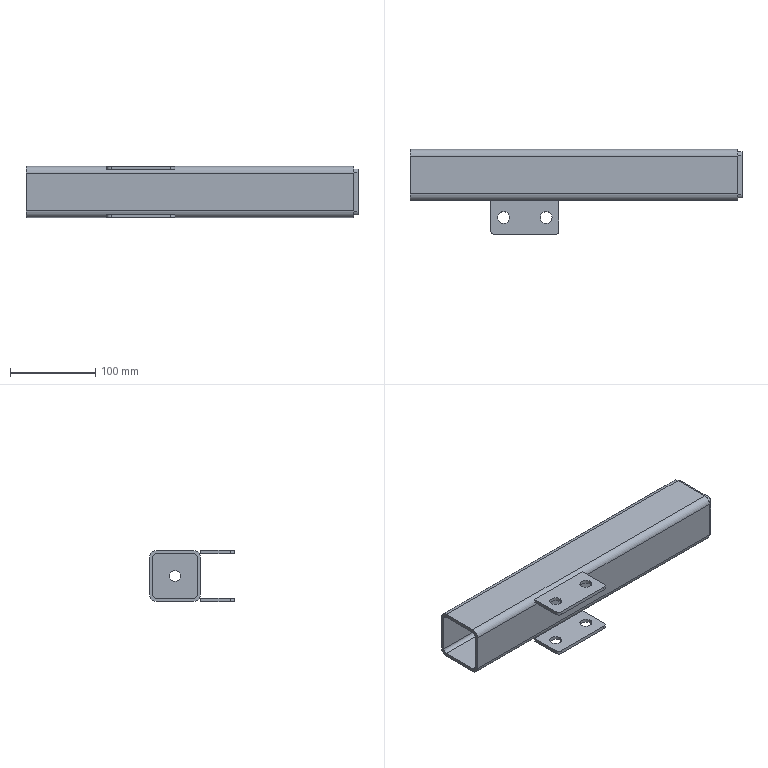Part | SolidWorks | features ICE 3, HoleWzd 1, MirrorSolid 1, WeldMemberFeat 1, WeldmentFeature 1 | 4 solids | 56 faces | box 390 x 100 x 60 mm | volume 365741 mm3 | cylinder 28 | plane 28 | commonest cylinder face diameters 8 x8 14 x8 10 x4 16 x4 9 x2 13 x2